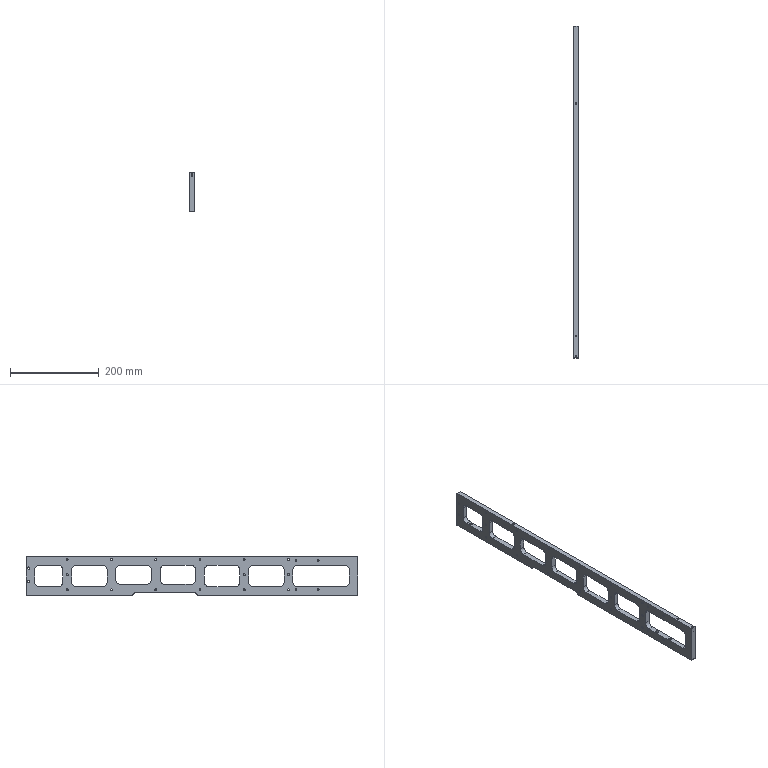Part | 1 solid | 105 faces | box 11 x 750 x 88 mm | volume 414841 mm3 | cylinder 63 | plane 42 | commonest cylinder face diameters 20 x28 4.2 x17 5.02 x5 2 x4 10 x4 6.5 x3